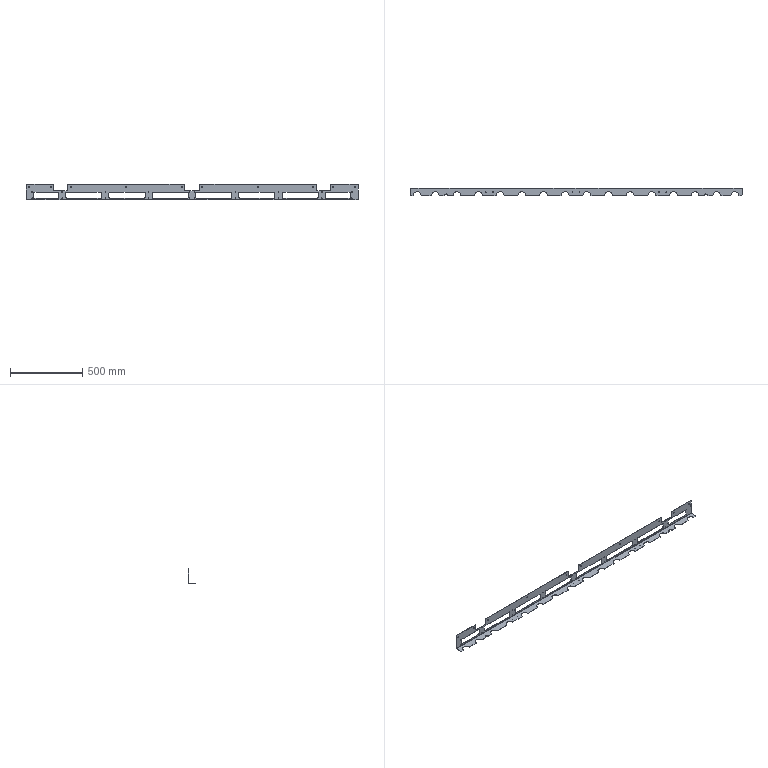Part | STEP file | DCV-000-035-2300L | 1 solid | 334 faces | box 2300 x 51.1 x 110 mm | volume 413040 mm3 | cylinder 260 | plane 74 | commonest cylinder face diameters 10 x96 4 x72 3.242 x52 7 x20 54 x16 25 x2